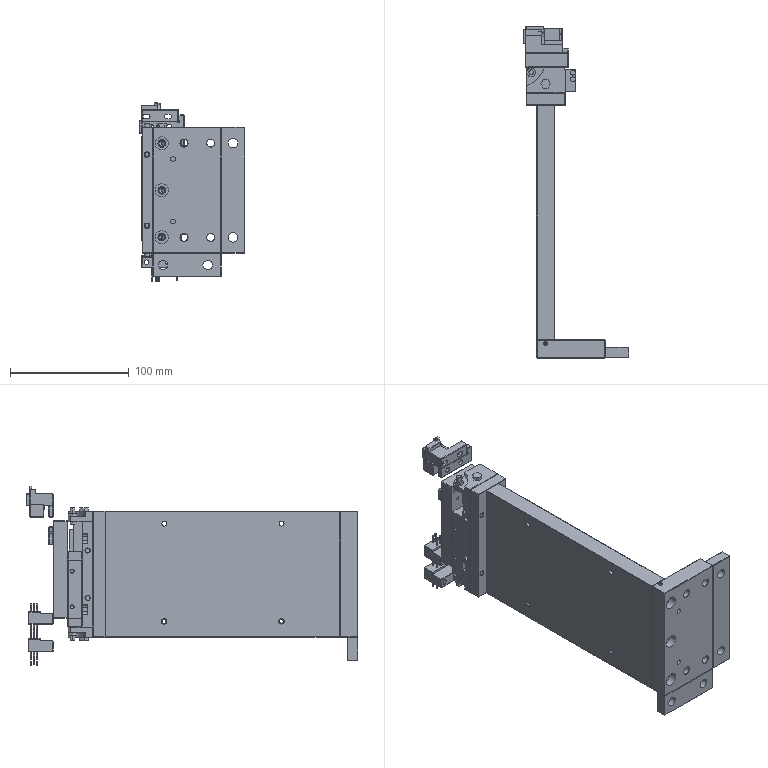Part | NX | 42 solids | 1280 faces | box 89 x 279.82 x 150.452 mm | volume 587217 mm3 | plane 629 | cylinder 503 | cone 148 | commonest cylinder face diameters 4 x57 1.31 x48 5 x32 1.35 x28 3 x26 4.5 x26